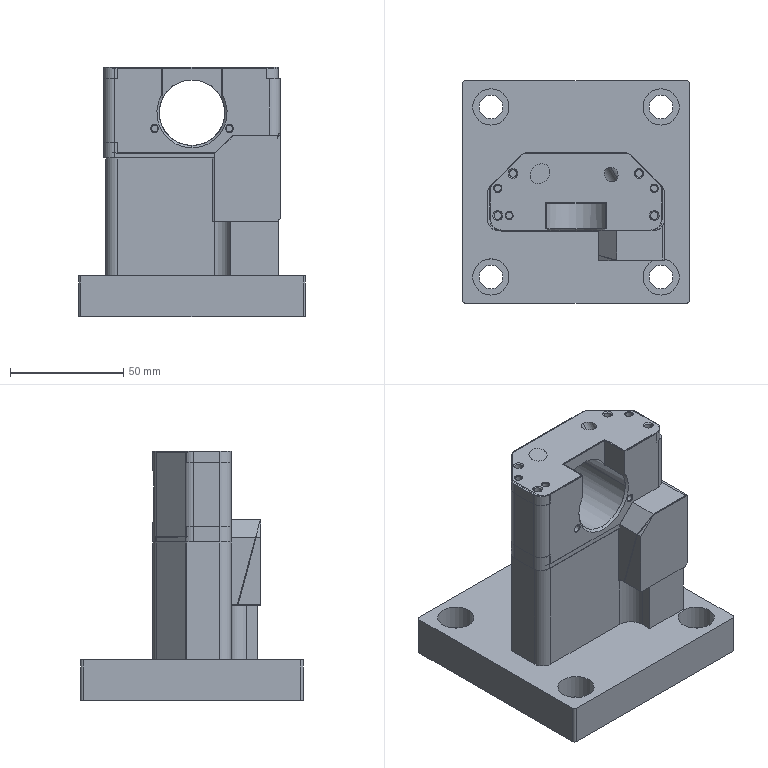NC program | NX | posted with a generic post | part box 100 x 98 x 110 mm
Lines 1 to 968 of 3149:
N10 G17 G21 G94 G90
(FLOOR_WALL_2_COPY , TOOL : D8-25-D8-60-3T-ROUGH)
N12 T26 M6
N14 G54
N16 G17 G0 G90 X-38.683 Y6.192 B0. C0. S4500 M3
N18 G43 Z33. H26
N20 Z3.
N22 G94 G1 Z0. F1000.
N24 Y5.95
N26 G3 X-36.683 Y3.95 R2.
N28 G1 X-11.224
N30 X-6.3 Y-0.974
N32 Y-1.225
N34 X-41.7
N36 Y-6.4
N38 X-6.3
N40 Y-11.575
N42 X-41.7
N44 Y-16.75
N46 X-6.3
N48 G3 X-4.3 Y-14.75 R2.
N50 G1 X-3.3
N52 Z3.
N54 G0 Z33.
(PLANAR_MILL_25_COPY , TOOL : D8-25-D8-60-3T-ROUGH)
N56 X-46.256 Y-5.057 S6500
N58 Z30.
N60 Z-10.95
N62 G1 Z-13.95 F1200.
N64 X-40.599 Y0.599
N66 X-32.049 Y9.149
N68 G2 X-29.15 Y10.35 R4.1
N70 G1 X-18.756
N72 G2 X-15.857 Y9.149 R4.1
N74 G1 X-7.101 Y0.393
N76 G2 X-5.9 Y-2.506 R4.1
N78 G1 Y-27.992
N80 Y-35.992
N82 Z-10.95
N84 G0 Z30.
N86 X-46.256 Y-5.057
N88 Z-24.9
N90 G1 Z-27.9
N92 X-40.599 Y0.599
N94 X-32.049 Y9.149
N96 G2 X-29.15 Y10.35 R4.1
N98 G1 X-18.756
N100 G2 X-15.857 Y9.149 R4.1
N102 G1 X-7.101 Y0.393
N104 G2 X-5.9 Y-2.506 R4.1
N106 G1 Y-27.992
N108 Y-35.992
N110 Z-24.9
N112 G0 Z30.
(PLANAR_MILL_25_COPY_COPY , TOOL : D8-25-D8-60-3T-ROUGH)
N114 X-46.256 Y-5.057
N116 Z20.
N118 Z-25.95
N120 G1 Z-28.95
N122 X-40.599 Y0.599
N124 X-32.049 Y9.149
N126 G2 X-29.15 Y10.35 R4.1
N128 G1 X-18.756
N130 G2 X-15.857 Y9.149 R4.1
N132 G1 X-7.101 Y0.393
N134 G2 X-5.9 Y-2.506 R4.1
N136 G1 Y-27.992
N138 Y-35.992
N140 Z-25.95
N142 G0 Z20.
N144 X-46.256 Y-5.057
N146 Z-26.9
N148 G1 Z-29.9
N150 X-40.599 Y0.599
N152 X-32.049 Y9.149
N154 G2 X-29.15 Y10.35 R4.1
N156 G1 X-18.756
N158 G2 X-15.857 Y9.149 R4.1
N160 G1 X-7.101 Y0.393
N162 G2 X-5.9 Y-2.506 R4.1
N164 G1 Y-27.992
N166 Y-35.992
N168 Z-26.9
N170 G0 Z20.
(FLOOR_WALL_1 , TOOL : D8-25-D8-60-3T-ROUGH)
N172 Z30.2
N174 X16.638 Y-23.95
N176 Z-25.3
N178 G1 Z-28.3 F1500.
N180 Y-16.95
N182 G3 X14.638 Y-14.95 R2.
N184 G1 X-5.8
N186 Y-0.767
N188 X-17.017 Y10.45
N190 X-26.647
N192 X-26.047 Y11.05
N194 X26.047
N196 X35.7 Y1.397
N198 Y-12.25
N200 G2 X33. Y-14.95 R2.7
N202 G1 X14.638
N204 Y-8.95
N206 X0.2
N208 Y-0.767
N210 G3 X-1.557 Y3.476 R6.
N212 G1 X-3.131 Y5.05
N214 X-7.198 Y6.734
N216 X-3.131 Y5.05
N218 X23.562
N220 X29.7 Y-1.088
N222 Y-8.95
N224 X14.638
N226 Y-2.95
N228 X6.2
N230 Y-0.95
N232 X21.077
N234 X23.077 Y-2.95
N236 X14.638
N238 X13.638
N240 G3 X11.638 Y-4.95 R2.
N242 G1 Z-25.3
N244 G0 Z30.2
N246 X16.638 Y-23.95
N248 Z-26.1
N250 G1 Z-29.1
N252 Y-16.95
N254 G3 X14.638 Y-14.95 R2.
N256 G1 X-5.8
N258 Y-0.767
N260 X-17.017 Y10.45
N262 X-26.647
N264 X-26.047 Y11.05
N266 X26.047
N268 X35.7 Y1.397
N270 Y-12.25
N272 G2 X33. Y-14.95 R2.7
N274 G1 X14.638
N276 Y-8.95
N278 X0.2
N280 Y-0.767
N282 G3 X-1.557 Y3.476 R6.
N284 G1 X-3.131 Y5.05
N286 X-7.198 Y6.734
N288 X-3.131 Y5.05
N290 X23.562
N292 X29.7 Y-1.088
N294 Y-8.95
N296 X14.638
N298 Y-2.95
N300 X6.2
N302 Y-0.95
N304 X21.077
N306 X23.077 Y-2.95
N308 X14.638
N310 X13.638
N312 G3 X11.638 Y-4.95 R2.
N314 G1 Z-26.1
N316 G0 Z30.2
N318 X16.638 Y-23.95
N320 Z-26.9
N322 G1 Z-29.9
N324 Y-16.95
N326 G3 X14.638 Y-14.95 R2.
N328 G1 X-5.8
N330 Y-0.767
N332 X-17.017 Y10.45
N334 X-26.647
N336 X-26.047 Y11.05
N338 X26.047
N340 X35.7 Y1.397
N342 Y-12.25
N344 G2 X33. Y-14.95 R2.7
N346 G1 X14.638
N348 Y-8.95
N350 X0.2
N352 Y-0.767
N354 G3 X-1.557 Y3.476 R6.
N356 G1 X-3.131 Y5.05
N358 X-7.198 Y6.734
N360 X-3.131 Y5.05
N362 X23.562
N364 X29.7 Y-1.088
N366 Y-8.95
N368 X14.638
N370 Y-2.95
N372 X6.2
N374 Y-0.95
N376 X21.077
N378 X23.077 Y-2.95
N380 X14.638
N382 X13.638
N384 G3 X11.638 Y-4.95 R2.
N386 G1 Z-26.9
N388 G0 Z30.2
(FLOOR_WALL_1_COPY_3 , TOOL : D8-25-D8-60-3T-ROUGH)
N390 X-7.997 Y8.25
N392 Z30.1
N394 Z-24.4
N396 G1 Z-27.4
N398 Y11.25
N400 Y21.25
N402 X-2.665
N404 Y11.25
N406 X2.668
N408 Y21.25
N410 X8.
N412 Y11.25
N414 Y8.25
N416 Z-24.4
N418 G0 Z30.1
N420 X-7.997 Y8.15
N422 Z-25.2
N424 G1 Z-28.2
N426 Y11.25
N428 Y21.25
N430 X-2.665
N432 Y11.25
N434 X2.668
N436 Y21.25
N438 X8.
N440 Y11.25
N442 Y8.15
N444 Z-25.2
N446 G0 Z30.1
N448 X-7.997
N450 Z-26.
N452 G1 Z-29.
N454 Y11.25
N456 Y21.25
N458 X-2.665
N460 Y11.25
N462 X2.668
N464 Y21.25
N466 X8.
N468 Y11.25
N470 Y8.15
N472 Z-26.
N474 G0 Z30.1
(PLANAR_MILL_24 , TOOL : D8-25-D8-60-3T-ROUGH)
N476 X-32. Y19.25
N478 Z2.1
N480 Z-24.9
N482 G1 Z-27.9
N484 X-24.
N486 X24.
N488 X32.
N490 Z-24.9
N492 G0 Z2.1
(PLANAR_MILL_11 , TOOL : D8-25-D8-60-3T-ROUGH)
N494 X28.805 Y-7.356
N496 Z0.
N498 Z-28.
N500 G1 X29.189 Y-6.821 Z-28.017
N502 X29.525 Y-5.711 Z-28.048
N504 Y-4.789 Z-28.072
N506 X29.189 Y-3.679 Z-28.102
N508 X28.514 Y-2.736 Z-28.132
N510 X27.571 Y-2.061 Z-28.163
N512 X26.461 Y-1.725 Z-28.193
N514 X25.539 Z-28.217
N516 X24.429 Y-2.061 Z-28.248
N518 X23.486 Y-2.736 Z-28.278
N520 X22.811 Y-3.679 Z-28.308
N522 X22.475 Y-4.789 Z-28.339
N524 Y-5.711 Z-28.363
N526 X22.811 Y-6.821 Z-28.393
N528 X23.486 Y-7.764 Z-28.424
N530 X24.429 Y-8.439 Z-28.454
N532 X25.539 Y-8.775 Z-28.484
N534 X26.461 Z-28.509
N536 X27.571 Y-8.439 Z-28.539
N538 X28.514 Y-7.764 Z-28.569
N540 X29.189 Y-6.821 Z-28.6
N542 X29.525 Y-5.711 Z-28.63
N544 Y-4.789 Z-28.654
N546 X29.189 Y-3.679 Z-28.685
N548 X28.514 Y-2.736 Z-28.715
N550 X27.571 Y-2.061 Z-28.745
N552 X26.461 Y-1.725 Z-28.776
N554 X25.539 Z-28.8
N556 X24.429 Y-2.061 Z-28.83
N558 X23.486 Y-2.736 Z-28.861
N560 X22.811 Y-3.679 Z-28.891
N562 X22.475 Y-4.789 Z-28.921
N564 Y-5.711 Z-28.945
N566 X22.811 Y-6.821 Z-28.976
N568 X23.486 Y-7.764 Z-29.006
N570 X24.429 Y-8.439 Z-29.037
N572 X25.539 Y-8.775 Z-29.067
N574 X26.461 Z-29.091
N576 X27.571 Y-8.439 Z-29.121
N578 X28.514 Y-7.764 Z-29.152
N580 X29.189 Y-6.821 Z-29.182
N582 X29.525 Y-5.711 Z-29.213
N584 Y-4.789 Z-29.237
N586 X29.189 Y-3.679 Z-29.267
N588 X28.514 Y-2.736 Z-29.297
N590 X27.571 Y-2.061 Z-29.328
N592 X26.461 Y-1.725 Z-29.358
N594 X25.539 Z-29.382
N596 X24.429 Y-2.061 Z-29.413
N598 X23.486 Y-2.736 Z-29.443
N600 X22.811 Y-3.679 Z-29.473
N602 X22.475 Y-4.789 Z-29.504
N604 Y-5.711 Z-29.528
N606 X22.811 Y-6.821 Z-29.558
N608 X23.486 Y-7.764 Z-29.589
N610 X24.429 Y-8.439 Z-29.619
N612 X25.539 Y-8.775 Z-29.649
N614 X26.461 Z-29.674
N616 X27.571 Y-8.439 Z-29.704
N618 X28.514 Y-7.764 Z-29.734
N620 X29.189 Y-6.821 Z-29.765
N622 X29.525 Y-5.711 Z-29.795
N624 Y-4.789 Z-29.819
N626 X29.189 Y-3.679 Z-29.849
N628 X28.514 Y-2.736 Z-29.88
N630 X27.571 Y-2.061 Z-29.91
N632 X26.461 Y-1.725 Z-29.941
N634 X25.539 Z-29.965
N636 X24.429 Y-2.061 Z-29.995
N638 X23.486 Y-2.736 Z-30.025
N640 X22.811 Y-3.679 Z-30.056
N642 X22.475 Y-4.789 Z-30.086
N644 Y-5.711 Z-30.11
N646 X22.811 Y-6.821 Z-30.141
N648 X23.486 Y-7.764 Z-30.171
N650 X24.429 Y-8.439 Z-30.201
N652 X25.539 Y-8.775 Z-30.232
N654 X26.461 Z-30.256
N656 X27.571 Y-8.439 Z-30.286
N658 X28.514 Y-7.764 Z-30.317
N660 X29.189 Y-6.821 Z-30.347
N662 X29.525 Y-5.711 Z-30.377
N664 Y-4.789 Z-30.402
N666 X29.189 Y-3.679 Z-30.432
N668 X28.514 Y-2.736 Z-30.462
N670 X27.571 Y-2.061 Z-30.493
N672 X26.461 Y-1.725 Z-30.523
N674 X25.539 Z-30.547
N676 X24.429 Y-2.061 Z-30.578
N678 X23.486 Y-2.736 Z-30.608
N680 X22.811 Y-3.679 Z-30.638
N682 X22.475 Y-4.789 Z-30.669
N684 Y-5.711 Z-30.693
N686 X22.811 Y-6.821 Z-30.723
N688 X23.486 Y-7.764 Z-30.754
N690 X24.429 Y-8.439 Z-30.784
N692 X25.539 Y-8.775 Z-30.814
N694 X26.461 Z-30.838
N696 X27.571 Y-8.439 Z-30.869
N698 X28.514 Y-7.764 Z-30.899
N700 X29.189 Y-6.821 Z-30.93
N702 X29.525 Y-5.711 Z-30.96
N704 Y-4.789 Z-30.984
N706 X29.189 Y-3.679 Z-31.014
N708 X28.514 Y-2.736 Z-31.045
N710 X27.571 Y-2.061 Z-31.075
N712 X26.461 Y-1.725 Z-31.106
N714 X25.539 Z-31.13
N716 X24.429 Y-2.061 Z-31.16
N718 X23.486 Y-2.736 Z-31.19
N720 X22.811 Y-3.679 Z-31.221
N722 X22.475 Y-4.789 Z-31.251
N724 Y-5.711 Z-31.275
N726 X22.811 Y-6.821 Z-31.306
N728 X23.486 Y-7.764 Z-31.336
N730 X24.429 Y-8.439 Z-31.366
N732 X25.539 Y-8.775 Z-31.397
N734 X26.461 Z-31.421
N736 X27.571 Y-8.439 Z-31.451
N738 X28.514 Y-7.764 Z-31.482
N740 X29.189 Y-6.821 Z-31.512
N742 X29.525 Y-5.711 Z-31.542
N744 Y-4.789 Z-31.566
N746 X29.189 Y-3.679 Z-31.597
N748 X28.514 Y-2.736 Z-31.627
N750 X27.571 Y-2.061 Z-31.658
N752 X26.461 Y-1.725 Z-31.688
N754 X25.539 Z-31.712
N756 X24.429 Y-2.061 Z-31.742
N758 X23.486 Y-2.736 Z-31.773
N760 X22.811 Y-3.679 Z-31.803
N762 X22.475 Y-4.789 Z-31.834
N764 Y-5.711 Z-31.858
N766 X22.811 Y-6.821 Z-31.888
N768 X23.486 Y-7.764 Z-31.918
N770 X24.429 Y-8.439 Z-31.949
N772 X25.539 Y-8.775 Z-31.979
N774 X26.461 Z-32.003
N776 X27.571 Y-8.439 Z-32.034
N778 X28.514 Y-7.764 Z-32.064
N780 X29.189 Y-6.821 Z-32.094
N782 X29.525 Y-5.711 Z-32.125
N784 Y-4.789 Z-32.149
N786 X29.189 Y-3.679 Z-32.179
N788 X28.514 Y-2.736 Z-32.21
N790 X27.571 Y-2.061 Z-32.24
N792 X26.461 Y-1.725 Z-32.27
N794 X25.539 Z-32.295
N796 X24.429 Y-2.061 Z-32.325
N798 X23.486 Y-2.736 Z-32.355
N800 X22.811 Y-3.679 Z-32.386
N802 X22.475 Y-4.789 Z-32.416
N804 Y-5.711 Z-32.44
N806 X22.811 Y-6.821 Z-32.471
N808 X23.486 Y-7.764 Z-32.501
N810 X24.429 Y-8.439 Z-32.531
N812 X25.539 Y-8.775 Z-32.562
N814 X26.461 Z-32.586
N816 X27.571 Y-8.439 Z-32.616
N818 X28.514 Y-7.764 Z-32.647
N820 X29.189 Y-6.821 Z-32.677
N822 X29.525 Y-5.711 Z-32.707
N824 Y-4.789 Z-32.731
N826 X29.189 Y-3.679 Z-32.762
N828 X28.514 Y-2.736 Z-32.792
N830 X27.571 Y-2.061 Z-32.822
N832 X26.461 Y-1.725 Z-32.853
N834 X25.539 Z-32.877
N836 X24.429 Y-2.061 Z-32.907
N838 X23.486 Y-2.736 Z-32.938
N840 X22.811 Y-3.679 Z-32.968
N842 X22.475 Y-4.789 Z-32.998
N844 Y-5.711 Z-33.023
N846 X22.811 Y-6.821 Z-33.053
N848 X23.486 Y-7.764 Z-33.083
N850 X24.429 Y-8.439 Z-33.114
N852 X25.539 Y-8.775 Z-33.144
N854 X26.461 Z-33.168
N856 X27.571 Y-8.439 Z-33.199
N858 X28.514 Y-7.764 Z-33.229
N860 X29.189 Y-6.821 Z-33.259
N862 X29.525 Y-5.711 Z-33.29
N864 Y-4.789 Z-33.314
N866 X29.189 Y-3.679 Z-33.344
N868 X28.514 Y-2.736 Z-33.375
N870 X27.571 Y-2.061 Z-33.405
N872 X26.461 Y-1.725 Z-33.435
N874 X25.539 Z-33.459
N876 X24.429 Y-2.061 Z-33.49
N878 X23.486 Y-2.736 Z-33.52
N880 X22.811 Y-3.679 Z-33.551
N882 X22.475 Y-4.789 Z-33.581
N884 Y-5.711 Z-33.605
N886 X22.811 Y-6.821 Z-33.635
N888 X23.486 Y-7.764 Z-33.666
N890 X24.429 Y-8.439 Z-33.696
N892 X25.539 Y-8.775 Z-33.727
N894 X26.461 Z-33.751
N896 X27.571 Y-8.439 Z-33.781
N898 X28.514 Y-7.764 Z-33.811
N900 X29.189 Y-6.821 Z-33.842
N902 X29.525 Y-5.711 Z-33.872
N904 Y-4.789 Z-33.896
N906 X29.189 Y-3.679 Z-33.927
N908 X28.514 Y-2.736 Z-33.957
N910 X27.571 Y-2.061 Z-33.987
N912 X26.461 Y-1.725 Z-34.018
N914 X25.539 Z-34.042
N916 X24.429 Y-2.061 Z-34.072
N918 X23.486 Y-2.736 Z-34.103
N920 X22.811 Y-3.679 Z-34.133
N922 X22.475 Y-4.789 Z-34.163
N924 Y-5.711 Z-34.188
N926 X22.811 Y-6.821 Z-34.218
N928 X23.486 Y-7.764 Z-34.248
N930 X24.429 Y-8.439 Z-34.279
N932 X25.539 Y-8.775 Z-34.309
N934 X26.461 Z-34.333
N936 X27.571 Y-8.439 Z-34.364
N938 X28.514 Y-7.764 Z-34.394
N940 X29.189 Y-6.821 Z-34.424
N942 X29.525 Y-5.711 Z-34.455
N944 Y-4.789 Z-34.479
N946 X29.189 Y-3.679 Z-34.509
N948 X28.514 Y-2.736 Z-34.539
N950 X27.571 Y-2.061 Z-34.57
N952 X26.461 Y-1.725 Z-34.6
N954 X25.539 Z-34.624
N956 X24.429 Y-2.061 Z-34.655
N958 X23.486 Y-2.736 Z-34.685
N960 X22.811 Y-3.679 Z-34.715
N962 X22.475 Y-4.789 Z-34.746
N964 Y-5.711 Z-34.77
N966 X22.811 Y-6.821 Z-34.8
N968 X23.486 Y-7.764 Z-34.831
N970 X24.429 Y-8.439 Z-34.861
N972 X25.539 Y-8.775 Z-34.891
N974 X26.461 Z-34.916
N976 X27.571 Y-8.439 Z-34.946
N978 X28.514 Y-7.764 Z-34.976
N980 X29.189 Y-6.821 Z-35.007
N982 X29.525 Y-5.711 Z-35.037
N984 Y-4.789 Z-35.061
N986 X29.189 Y-3.679 Z-35.092
N988 X28.514 Y-2.736 Z-35.122
N990 X27.571 Y-2.061 Z-35.152
N992 X26.461 Y-1.725 Z-35.183
N994 X25.539 Z-35.207
N996 X24.429 Y-2.061 Z-35.237
N998 X23.486 Y-2.736 Z-35.268
N1000 X22.811 Y-3.679 Z-35.298
N1002 X22.475 Y-4.789 Z-35.328
N1004 Y-5.711 Z-35.352
N1006 X22.811 Y-6.821 Z-35.383
N1008 X23.486 Y-7.764 Z-35.413
N1010 X24.429 Y-8.439 Z-35.444
N1012 X25.539 Y-8.775 Z-35.474
N1014 X26.461 Z-35.498
N1016 X27.571 Y-8.439 Z-35.528
N1018 X28.514 Y-7.764 Z-35.559
N1020 X29.189 Y-6.821 Z-35.589
N1022 X29.525 Y-5.711 Z-35.62
N1024 Y-4.789 Z-35.644
N1026 X29.189 Y-3.679 Z-35.674
N1028 X28.514 Y-2.736 Z-35.704
N1030 X27.571 Y-2.061 Z-35.735
N1032 X26.461 Y-1.725 Z-35.765
N1034 X25.539 Z-35.789
N1036 X24.429 Y-2.061 Z-35.82
N1038 X23.486 Y-2.736 Z-35.85
N1040 X22.811 Y-3.679 Z-35.88
N1042 X22.475 Y-4.789 Z-35.911
N1044 Y-5.711 Z-35.935
N1046 X22.811 Y-6.821 Z-35.965
N1048 X23.486 Y-7.764 Z-35.996
N1050 X24.429 Y-8.439 Z-36.026
N1052 X25.539 Y-8.775 Z-36.056
N1054 X26.461 Z-36.081
N1056 X27.571 Y-8.439 Z-36.111
N1058 X28.514 Y-7.764 Z-36.141
N1060 X29.189 Y-6.821 Z-36.172
N1062 X29.525 Y-5.711 Z-36.202
N1064 Y-4.789 Z-36.226
N1066 X29.189 Y-3.679 Z-36.256
N1068 X28.514 Y-2.736 Z-36.287
N1070 X27.571 Y-2.061 Z-36.317
N1072 X26.461 Y-1.725 Z-36.348
N1074 X25.539 Z-36.372
N1076 X24.429 Y-2.061 Z-36.402
N1078 X23.486 Y-2.736 Z-36.432
N1080 X22.811 Y-3.679 Z-36.463
N1082 X22.475 Y-4.789 Z-36.493
N1084 Y-5.711 Z-36.517
N1086 X22.811 Y-6.821 Z-36.548
N1088 X23.486 Y-7.764 Z-36.578
N1090 X24.429 Y-8.439 Z-36.608
N1092 X25.539 Y-8.775 Z-36.639
N1094 X26.461 Z-36.663
N1096 X27.571 Y-8.439 Z-36.693
N1098 X28.514 Y-7.764 Z-36.724
N1100 X29.189 Y-6.821 Z-36.754
N1102 X29.525 Y-5.711 Z-36.784
N1104 Y-4.789 Z-36.809
N1106 X29.189 Y-3.679 Z-36.839
N1108 X28.514 Y-2.736 Z-36.869
N1110 X27.571 Y-2.061 Z-36.9
N1112 X26.461 Y-1.725 Z-36.93
N1114 X25.539 Z-36.954
N1116 X24.429 Y-2.061 Z-36.985
N1118 X23.486 Y-2.736 Z-37.015
N1120 X22.811 Y-3.679 Z-37.045
N1122 X22.475 Y-4.789 Z-37.076
N1124 Y-5.711 Z-37.1
N1126 X22.811 Y-6.821 Z-37.13
N1128 X23.486 Y-7.764 Z-37.161
N1130 X24.429 Y-8.439 Z-37.191
N1132 X25.539 Y-8.775 Z-37.221
N1134 X26.461 Z-37.245
N1136 X27.571 Y-8.439 Z-37.276
N1138 X28.514 Y-7.764 Z-37.306
N1140 X29.189 Y-6.821 Z-37.337
N1142 X29.525 Y-5.711 Z-37.367
N1144 Y-4.789 Z-37.391
N1146 X29.189 Y-3.679 Z-37.421
N1148 X28.514 Y-2.736 Z-37.452
N1150 X27.571 Y-2.061 Z-37.482
N1152 X26.461 Y-1.725 Z-37.513
N1154 X25.539 Z-37.537
N1156 X24.429 Y-2.061 Z-37.567
N1158 X23.486 Y-2.736 Z-37.597
N1160 X22.811 Y-3.679 Z-37.628
N1162 X22.475 Y-4.789 Z-37.658
N1164 Y-5.711 Z-37.682
N1166 X22.811 Y-6.821 Z-37.713
N1168 X23.486 Y-7.764 Z-37.743
N1170 X24.429 Y-8.439 Z-37.773
N1172 X25.539 Y-8.775 Z-37.804
N1174 X26.461 Z-37.828
N1176 X27.571 Y-8.439 Z-37.858
N1178 X28.514 Y-7.764 Z-37.889
N1180 X29.189 Y-6.821 Z-37.919
N1182 X29.525 Y-5.711 Z-37.949
N1184 Y-4.789 Z-37.973
N1186 X29.189 Y-3.679 Z-38.004
N1188 X28.514 Y-2.736 Z-38.034
N1190 X27.571 Y-2.061 Z-38.065
N1192 X26.461 Y-1.725 Z-38.095
N1194 X25.539 Z-38.119
N1196 X24.429 Y-2.061 Z-38.149
N1198 X23.486 Y-2.736 Z-38.18
N1200 X22.811 Y-3.679 Z-38.21
N1202 X22.475 Y-4.789 Z-38.241
N1204 Y-5.711 Z-38.265
N1206 X22.811 Y-6.821 Z-38.295
N1208 X23.486 Y-7.764 Z-38.325
N1210 X24.429 Y-8.439 Z-38.356
N1212 X25.539 Y-8.775 Z-38.386
N1214 X26.461 Z-38.41
N1216 X27.571 Y-8.439 Z-38.441
N1218 X28.514 Y-7.764 Z-38.471
N1220 X29.189 Y-6.821 Z-38.501
N1222 X29.525 Y-5.711 Z-38.532
N1224 Y-4.789 Z-38.556
N1226 X29.189 Y-3.679 Z-38.586
N1228 X28.514 Y-2.736 Z-38.617
N1230 X27.571 Y-2.061 Z-38.647
N1232 X26.461 Y-1.725 Z-38.677
N1234 X25.539 Z-38.702
N1236 X24.429 Y-2.061 Z-38.732
N1238 X23.486 Y-2.736 Z-38.762
N1240 X22.811 Y-3.679 Z-38.793
N1242 X22.475 Y-4.789 Z-38.823
N1244 Y-5.711 Z-38.847
N1246 X22.811 Y-6.821 Z-38.878
N1248 X23.486 Y-7.764 Z-38.908
N1250 X24.429 Y-8.439 Z-38.938
N1252 X25.539 Y-8.775 Z-38.969
N1254 X26.461 Z-38.993
N1256 X27.571 Y-8.439 Z-39.023
N1258 X28.514 Y-7.764 Z-39.054
N1260 X29.189 Y-6.821 Z-39.084
N1262 X29.525 Y-5.711 Z-39.114
N1264 Y-4.789 Z-39.138
N1266 X29.189 Y-3.679 Z-39.169
N1268 X28.514 Y-2.736 Z-39.199
N1270 X27.571 Y-2.061 Z-39.229
N1272 X26.461 Y-1.725 Z-39.26
N1274 X25.539 Z-39.284
N1276 X24.429 Y-2.061 Z-39.314
N1278 X23.486 Y-2.736 Z-39.345
N1280 X22.811 Y-3.679 Z-39.375
N1282 X22.475 Y-4.789 Z-39.405
N1284 Y-5.711 Z-39.43
N1286 X22.811 Y-6.821 Z-39.46
N1288 X23.486 Y-7.764 Z-39.49
N1290 X24.429 Y-8.439 Z-39.521
N1292 X25.539 Y-8.775 Z-39.551
N1294 X26.461 Z-39.575
N1296 X27.571 Y-8.439 Z-39.606
N1298 X28.514 Y-7.764 Z-39.636
N1300 X29.189 Y-6.821 Z-39.666
N1302 X29.525 Y-5.711 Z-39.697
N1304 Y-4.789 Z-39.721
N1306 X29.189 Y-3.679 Z-39.751
N1308 X28.514 Y-2.736 Z-39.782
N1310 X27.571 Y-2.061 Z-39.812
N1312 X26.461 Y-1.725 Z-39.842
N1314 X25.539 Z-39.866
N1316 X24.429 Y-2.061 Z-39.897
N1318 X23.486 Y-2.736 Z-39.927
N1320 X22.811 Y-3.679 Z-39.958
N1322 X22.475 Y-4.789 Z-39.988
N1324 Y-5.25 Z-40.
N1326 G3 X26. Y-8.775 R3.525
N1328 X22.475 Y-5.25 R-3.525
N1330 G1 X26.475
N1332 Z-37.
N1334 G0 Z0.
(PLANAR_MILL_35 , TOOL : D8-25-D8-60-3T-ROUGH)
N1336 X44.1 Y4.279 S4500
N1338 Z-32.9
N1340 G1 Z-34.9 F800.
N1342 G3 X42.1 Y2.279 R2.
N1344 G1 Y-12.25
N1346 G2 X33. Y-21.35 R9.1
N1348 G3 X31. Y-23.35 R2.
N1350 G1 Z-32.9
N1352 G0 Z0.
(FLOOR_WALL_1_COPY_1_1 , TOOL : D8-25-D8-60-3T-ROUGH)
N1354 G3P2 X0. Y0. Z0. I0. J74.9748 K-39.9168
N1356 G53.1
N1358 X22.176 Y-36.663 Z55.558 S5500 H26
N1360 Z27.083
N1362 G1 Z24.083 F1200.
N1364 X18.977 Y-39.339
N1366 X-4.808 Y-59.239
N1368 X-8.388 Y-54.96
N1370 X18.763 Y-32.245
N1372 X15.183 Y-27.966
N1374 X-11.968 Y-50.681
N1376 X-15.548 Y-46.402
N1378 X11.603 Y-23.686
N1380 X8.023 Y-19.407
N1382 X-19.128 Y-42.123
N1384 X-22.708 Y-37.844
N1386 X4.443 Y-15.128
N1388 X0.863 Y-10.849
N1390 X-26.288 Y-33.564
N1392 X-28.589 Y-35.489
N1394 Z27.083
N1396 G0 Z28.558
N1398 X22.176 Y-36.663
N1400 Z25.608
N1402 G1 Z22.608
N1404 X18.977 Y-39.339
N1406 X-4.808 Y-59.239
N1408 X-8.388 Y-54.96
N1410 X18.763 Y-32.245
N1412 X15.183 Y-27.966
N1414 X-11.968 Y-50.681
N1416 X-15.548 Y-46.402
N1418 X11.603 Y-23.686
N1420 X8.023 Y-19.407
N1422 X-19.128 Y-42.123
N1424 X-22.708 Y-37.844
N1426 X4.443 Y-15.128
N1428 X0.863 Y-10.849
N1430 X-26.288 Y-33.564
N1432 X-28.589 Y-35.489
N1434 Z25.608
N1436 G0 Z28.558
N1438 X22.176 Y-36.663
N1440 Z24.133
N1442 G1 Z21.133
N1444 X18.977 Y-39.339
N1446 X-4.808 Y-59.239
N1448 X-8.388 Y-54.96
N1450 X18.763 Y-32.245
N1452 X15.183 Y-27.966
N1454 X-11.968 Y-50.681
N1456 X-15.548 Y-46.402
N1458 X11.603 Y-23.686
N1460 X8.023 Y-19.407
N1462 X-19.128 Y-42.123
N1464 X-22.708 Y-37.844
N1466 X4.443 Y-15.128
N1468 X0.863 Y-10.849
N1470 X-26.288 Y-33.564
N1472 X-28.589 Y-35.489
N1474 Z24.133
N1476 G0 Z28.558
N1478 X22.176 Y-36.663
N1480 Z22.658
N1482 G1 Z19.658
N1484 X18.977 Y-39.339
N1486 X-4.808 Y-59.239
N1488 X-8.388 Y-54.96
N1490 X18.763 Y-32.245
N1492 X15.183 Y-27.966
N1494 X-11.968 Y-50.681
N1496 X-15.548 Y-46.402
N1498 X11.603 Y-23.686
N1500 X8.023 Y-19.407
N1502 X-19.128 Y-42.123
N1504 X-22.708 Y-37.844
N1506 X4.443 Y-15.128
N1508 X0.863 Y-10.849
N1510 X-26.288 Y-33.564
N1512 X-28.589 Y-35.489
N1514 Z22.658
N1516 G0 Z55.558
(PLANAR_MILL_11_1 , TOOL : D8-25-D8-60-3T-ROUGH)
N1518 X2.854 Y-42.676 Z49.558 H26
N1520 Z20.558
N1522 G1 X3.394 Y-42.411 Z20.547
N1524 X4.276 Y-41.673 Z20.527
N1526 X5.165 Y-40.462 Z20.501
N1528 X5.696 Y-39.057 Z20.475
N1530 X5.829 Y-37.561 Z20.448
N1532 X5.555 Y-36.084 Z20.422
N1534 X4.893 Y-34.736 Z20.396
N1536 X4.155 Y-33.853 Z20.376
N1538 X2.944 Y-32.964 Z20.35
N1540 X1.539 Y-32.433 Z20.323
N1542 X0.043 Y-32.3 Z20.297
N1544 X-1.434 Y-32.574 Z20.271
N1546 X-2.782 Y-33.236 Z20.245
N1548 X-3.665 Y-33.974 Z20.225
N1550 X-4.554 Y-35.185 Z20.199
N1552 X-5.085 Y-36.59 Z20.172
N1554 X-5.218 Y-38.086 Z20.146
N1556 X-4.944 Y-39.563 Z20.12
N1558 X-4.282 Y-40.912 Z20.094
N1560 X-3.544 Y-41.794 Z20.074
N1562 X-2.333 Y-42.684 Z20.047
N1564 X-0.928 Y-43.214 Z20.021
N1566 X0.568 Y-43.347 Z19.995
N1568 X2.045 Y-43.073 Z19.969
N1570 X3.394 Y-42.411 Z19.942
N1572 X4.276 Y-41.673 Z19.922
N1574 X5.165 Y-40.462 Z19.896
N1576 X5.696 Y-39.057 Z19.87
N1578 X5.829 Y-37.561 Z19.844
N1580 X5.555 Y-36.084 Z19.818
N1582 X4.893 Y-34.736 Z19.791
N1584 X4.155 Y-33.853 Z19.771
N1586 X2.944 Y-32.964 Z19.745
N1588 X1.539 Y-32.433 Z19.719
N1590 X0.043 Y-32.3 Z19.693
N1592 X-1.434 Y-32.574 Z19.666
N1594 X-2.782 Y-33.236 Z19.64
N1596 X-3.665 Y-33.974 Z19.62
N1598 X-4.554 Y-35.185 Z19.594
N1600 X-5.085 Y-36.59 Z19.568
N1602 X-5.218 Y-38.086 Z19.541
N1604 X-4.944 Y-39.563 Z19.515
N1606 X-4.282 Y-40.912 Z19.489
N1608 X-3.544 Y-41.794 Z19.469
N1610 X-2.333 Y-42.684 Z19.443
N1612 X-0.928 Y-43.214 Z19.416
N1614 X0.568 Y-43.347 Z19.39
N1616 X2.045 Y-43.073 Z19.364
N1618 X3.394 Y-42.411 Z19.338
N1620 X4.276 Y-41.673 Z19.318
N1622 X5.165 Y-40.462 Z19.291
N1624 X5.696 Y-39.057 Z19.265
N1626 X5.829 Y-37.561 Z19.239
N1628 X5.555 Y-36.084 Z19.213
N1630 X4.893 Y-34.736 Z19.187
N1632 X4.155 Y-33.853 Z19.166
N1634 X2.944 Y-32.964 Z19.14
N1636 X1.539 Y-32.433 Z19.114
N1638 X0.043 Y-32.3 Z19.088
N1640 X-1.434 Y-32.574 Z19.062
N1642 X-2.782 Y-33.236 Z19.035
N1644 X-3.665 Y-33.974 Z19.015
N1646 X-4.554 Y-35.185 Z18.989
N1648 X-5.085 Y-36.59 Z18.963
N1650 X-5.218 Y-38.086 Z18.937
N1652 X-4.944 Y-39.563 Z18.91
N1654 X-4.282 Y-40.912 Z18.884
N1656 X-3.544 Y-41.794 Z18.864
N1658 X-2.333 Y-42.684 Z18.838
N1660 X-0.928 Y-43.214 Z18.812
N1662 X0.568 Y-43.347 Z18.785
N1664 X2.045 Y-43.073 Z18.759
N1666 X3.394 Y-42.411 Z18.733
N1668 X4.276 Y-41.673 Z18.713
N1670 X5.165 Y-40.462 Z18.687
N1672 X5.696 Y-39.057 Z18.661
N1674 X5.829 Y-37.561 Z18.634
N1676 X5.555 Y-36.084 Z18.608
N1678 X4.893 Y-34.736 Z18.582
N1680 X4.155 Y-33.853 Z18.562
N1682 X2.944 Y-32.964 Z18.536
N1684 X1.539 Y-32.433 Z18.509
N1686 X0.043 Y-32.3 Z18.483
N1688 X-1.434 Y-32.574 Z18.457
N1690 X-2.782 Y-33.236 Z18.431
N1692 X-3.665 Y-33.974 Z18.411
N1694 X-4.554 Y-35.185 Z18.384
N1696 X-5.085 Y-36.59 Z18.358
N1698 X-5.218 Y-38.086 Z18.332
N1700 X-4.944 Y-39.563 Z18.306
N1702 X-4.282 Y-40.912 Z18.279
N1704 X-3.544 Y-41.794 Z18.259
N1706 X-2.333 Y-42.684 Z18.233
N1708 X-0.928 Y-43.214 Z18.207
N1710 X0.568 Y-43.347 Z18.181
N1712 X2.045 Y-43.073 Z18.155
N1714 X3.394 Y-42.411 Z18.128
N1716 X4.276 Y-41.673 Z18.108
N1718 X5.165 Y-40.462 Z18.082
N1720 X5.696 Y-39.057 Z18.056
N1722 X5.829 Y-37.561 Z18.03
N1724 X5.555 Y-36.084 Z18.003
N1726 X4.893 Y-34.736 Z17.977
N1728 X4.155 Y-33.853 Z17.957
N1730 X2.944 Y-32.964 Z17.931
N1732 X1.539 Y-32.433 Z17.905
N1734 X0.043 Y-32.3 Z17.878
N1736 X-1.434 Y-32.574 Z17.852
N1738 X-2.782 Y-33.236 Z17.826
N1740 X-3.665 Y-33.974 Z17.806
N1742 X-4.554 Y-35.185 Z17.78
N1744 X-5.085 Y-36.59 Z17.753
N1746 X-5.218 Y-38.086 Z17.727
N1748 X-4.944 Y-39.563 Z17.701
N1750 X-4.282 Y-40.912 Z17.675
N1752 X-3.544 Y-41.794 Z17.655
N1754 X-2.333 Y-42.684 Z17.628
N1756 X-0.928 Y-43.214 Z17.602
N1758 X0.568 Y-43.347 Z17.576
N1760 X2.045 Y-43.073 Z17.55
N1762 X3.394 Y-42.411 Z17.524
N1764 X4.276 Y-41.673 Z17.503
N1766 X5.165 Y-40.462 Z17.477
N1768 X5.696 Y-39.057 Z17.451
N1770 X5.829 Y-37.561 Z17.425
N1772 X5.555 Y-36.084 Z17.399
N1774 X4.893 Y-34.736 Z17.372
N1776 X4.155 Y-33.853 Z17.352
N1778 X2.944 Y-32.964 Z17.326
N1780 X1.539 Y-32.433 Z17.3
N1782 X0.043 Y-32.3 Z17.274
N1784 X-1.434 Y-32.574 Z17.247
N1786 X-2.782 Y-33.236 Z17.221
N1788 X-3.665 Y-33.974 Z17.201
N1790 X-4.554 Y-35.185 Z17.175
N1792 X-5.085 Y-36.59 Z17.149
N1794 X-5.218 Y-38.086 Z17.122
N1796 X-4.944 Y-39.563 Z17.096
N1798 X-4.282 Y-40.912 Z17.07
N1800 X-3.544 Y-41.794 Z17.05
N1802 X-2.333 Y-42.684 Z17.024
N1804 X-0.928 Y-43.214 Z16.998
N1806 X0.568 Y-43.347 Z16.971
N1808 X2.045 Y-43.073 Z16.945
N1810 X3.394 Y-42.411 Z16.919
N1812 X4.276 Y-41.673 Z16.899
N1814 X5.165 Y-40.462 Z16.873
N1816 X5.696 Y-39.057 Z16.846
N1818 X5.829 Y-37.561 Z16.82
N1820 X5.555 Y-36.084 Z16.794
N1822 X4.893 Y-34.736 Z16.768
N1824 X4.155 Y-33.853 Z16.748
N1826 X2.944 Y-32.964 Z16.721
N1828 X1.539 Y-32.433 Z16.695
N1830 X0.043 Y-32.3 Z16.669
N1832 X-1.434 Y-32.574 Z16.643
N1834 X-2.782 Y-33.236 Z16.616
N1836 X-3.665 Y-33.974 Z16.596
N1838 X-4.554 Y-35.185 Z16.57
N1840 X-5.085 Y-36.59 Z16.544
N1842 X-5.218 Y-38.086 Z16.518
N1844 X-4.944 Y-39.563 Z16.492
N1846 X-4.282 Y-40.912 Z16.465
N1848 X-3.544 Y-41.794 Z16.445
N1850 X-2.333 Y-42.684 Z16.419
N1852 X-0.928 Y-43.214 Z16.393
N1854 X0.568 Y-43.347 Z16.367
N1856 X2.045 Y-43.073 Z16.34
N1858 X3.394 Y-42.411 Z16.314
N1860 X4.276 Y-41.673 Z16.294
N1862 X5.165 Y-40.462 Z16.268
N1864 X5.696 Y-39.057 Z16.242
N1866 X5.829 Y-37.561 Z16.215
N1868 X5.555 Y-36.084 Z16.189
N1870 X4.893 Y-34.736 Z16.163
N1872 X4.155 Y-33.853 Z16.143
N1874 X2.944 Y-32.964 Z16.117
N1876 X1.539 Y-32.433 Z16.09
N1878 X0.043 Y-32.3 Z16.064
N1880 X-1.434 Y-32.574 Z16.038